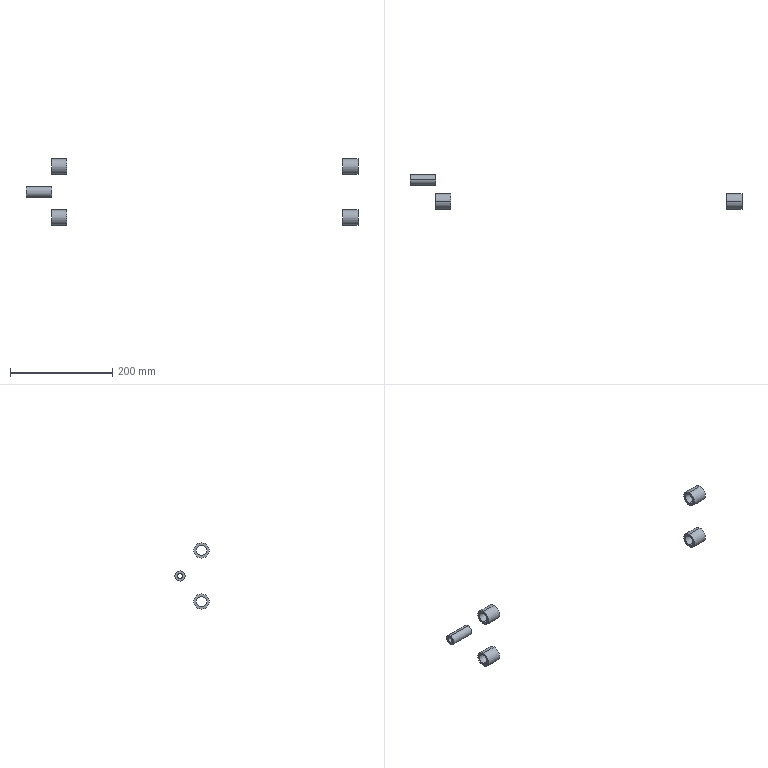Part | SolidWorks | features ICE 1, MirrorSolid 1, Revolution 1 | 5 solids | 30 faces | box 650 x 67 x 130 mm | volume 58905 mm3 | cylinder 20 | plane 10 | commonest cylinder face diameters 20 x10 30 x8 10 x2
STEP:
#1=CARTESIAN_POINT('',(-270.,0.,-10.));
#2=VERTEX_POINT('',#1);
#3=CARTESIAN_POINT('',(-270.,0.,10.));
#4=VERTEX_POINT('',#3);
#5=CARTESIAN_POINT('',(-270.,0.,0.));
#6=DIRECTION('',(-1.,0.,0.));
#7=DIRECTION('',(0.,0.,1.));
#8=AXIS2_PLACEMENT_3D('',#5,#6,#7);
#9=CIRCLE('',#8,10.);
#10=EDGE_CURVE('',#2,#4,#9,.T.);
#11=ORIENTED_EDGE('',*,*,#10,.F.);
#12=CARTESIAN_POINT('',(-300.,0.,-10.));
#13=VERTEX_POINT('',#12);
#14=CARTESIAN_POINT('',(-367.381,0.,-10.));
#15=DIRECTION('',(-1.,0.,0.));
#16=VECTOR('',#15,1000.);
#17=LINE('',#14,#16);
#18=EDGE_CURVE('',#2,#13,#17,.T.);
#19=ORIENTED_EDGE('',*,*,#18,.T.);
#20=CARTESIAN_POINT('',(-300.,0.,10.));
#21=VERTEX_POINT('',#20);
#22=CARTESIAN_POINT('',(-300.,0.,0.));
#23=DIRECTION('',(-1.,0.,0.));
#24=DIRECTION('',(0.,0.,1.));
#25=AXIS2_PLACEMENT_3D('',#22,#23,#24);
#26=CIRCLE('',#25,10.);
#27=EDGE_CURVE('',#13,#21,#26,.T.);
#28=ORIENTED_EDGE('',*,*,#27,.T.);
#29=CARTESIAN_POINT('',(-367.381,0.,10.));
#30=DIRECTION('',(-1.,0.,0.));
#31=VECTOR('',#30,1000.);
#32=LINE('',#29,#31);
#33=EDGE_CURVE('',#4,#21,#32,.T.);
#34=ORIENTED_EDGE('',*,*,#33,.F.);
#35=EDGE_LOOP('',(#11,#19,#28,#34));
#36=FACE_OUTER_BOUND('',#35,.T.);
#37=CARTESIAN_POINT('',(-367.381,0.,0.));
#38=DIRECTION('',(-1.,0.,0.));
#39=DIRECTION('',(0.,0.,1.));
#40=AXIS2_PLACEMENT_3D('',#37,#38,#39);
#41=CYLINDRICAL_SURFACE('',#40,10.);
#42=ADVANCED_FACE('',(#36),#41,.F.);
#43=CARTESIAN_POINT('',(-270.,0.,15.));
#44=VERTEX_POINT('',#43);
#45=CARTESIAN_POINT('',(-270.,0.,-15.));
#46=VERTEX_POINT('',#45);
#47=CARTESIAN_POINT('',(-270.,0.,0.));
#48=DIRECTION('',(-1.,0.,0.));
#49=DIRECTION('',(0.,0.,1.));
#50=AXIS2_PLACEMENT_3D('',#47,#48,#49);
#51=CIRCLE('',#50,15.);
#52=EDGE_CURVE('',#44,#46,#51,.T.);
#53=ORIENTED_EDGE('',*,*,#52,.T.);
#54=CARTESIAN_POINT('',(-300.,0.,-15.));
#55=VERTEX_POINT('',#54);
#56=CARTESIAN_POINT('',(-367.381,0.,-15.));
#57=DIRECTION('',(-1.,0.,0.));
#58=VECTOR('',#57,1000.);
#59=LINE('',#56,#58);
#60=EDGE_CURVE('',#46,#55,#59,.T.);
#61=ORIENTED_EDGE('',*,*,#60,.T.);
#62=CARTESIAN_POINT('',(-300.,0.,15.));
#63=VERTEX_POINT('',#62);
#64=CARTESIAN_POINT('',(-300.,0.,0.));
#65=DIRECTION('',(-1.,0.,0.));
#66=DIRECTION('',(0.,0.,1.));
#67=AXIS2_PLACEMENT_3D('',#64,#65,#66);
#68=CIRCLE('',#67,15.);
#69=EDGE_CURVE('',#63,#55,#68,.T.);
#70=ORIENTED_EDGE('',*,*,#69,.F.);
#71=CARTESIAN_POINT('',(-367.381,0.,15.));
#72=DIRECTION('',(-1.,0.,0.));
#73=VECTOR('',#72,1000.);
#74=LINE('',#71,#73);
#75=EDGE_CURVE('',#44,#63,#74,.T.);
#76=ORIENTED_EDGE('',*,*,#75,.F.);
#77=EDGE_LOOP('',(#53,#61,#70,#76));
#78=FACE_OUTER_BOUND('',#77,.T.);
#79=CARTESIAN_POINT('',(-367.381,0.,0.));
#80=DIRECTION('',(-1.,0.,0.));
#81=DIRECTION('',(0.,0.,1.));
#82=AXIS2_PLACEMENT_3D('',#79,#80,#81);
#83=CYLINDRICAL_SURFACE('',#82,15.);
#84=ADVANCED_FACE('',(#78),#83,.T.);
#85=ORIENTED_EDGE('',*,*,#60,.F.);
#86=CARTESIAN_POINT('',(-270.,0.,0.));
#87=DIRECTION('',(-1.,0.,0.));
#88=DIRECTION('',(0.,0.,1.));
#89=AXIS2_PLACEMENT_3D('',#86,#87,#88);
#90=CIRCLE('',#89,15.);
#91=EDGE_CURVE('',#46,#44,#90,.T.);
#92=ORIENTED_EDGE('',*,*,#91,.T.);
#93=ORIENTED_EDGE('',*,*,#75,.T.);
#94=CARTESIAN_POINT('',(-300.,0.,0.));
#95=DIRECTION('',(-1.,0.,0.));
#96=DIRECTION('',(0.,0.,1.));
#97=AXIS2_PLACEMENT_3D('',#94,#95,#96);
#98=CIRCLE('',#97,15.);
#99=EDGE_CURVE('',#55,#63,#98,.T.);
#100=ORIENTED_EDGE('',*,*,#99,.F.);
#101=EDGE_LOOP('',(#85,#92,#93,#100));
#102=FACE_OUTER_BOUND('',#101,.T.);
#103=CARTESIAN_POINT('',(-367.381,0.,0.));
#104=DIRECTION('',(-1.,0.,0.));
#105=DIRECTION('',(0.,0.,1.));
#106=AXIS2_PLACEMENT_3D('',#103,#104,#105);
#107=CYLINDRICAL_SURFACE('',#106,15.);
#108=ADVANCED_FACE('',(#102),#107,.T.);
#109=CARTESIAN_POINT('',(-300.,0.,0.));
#110=DIRECTION('',(-1.,0.,0.));
#111=DIRECTION('',(0.,0.,1.));
#112=AXIS2_PLACEMENT_3D('',#109,#110,#111);
#113=CIRCLE('',#112,10.);
#114=EDGE_CURVE('',#21,#13,#113,.T.);
#115=ORIENTED_EDGE('',*,*,#114,.F.);
#116=ORIENTED_EDGE('',*,*,#27,.F.);
#117=EDGE_LOOP('',(#115,#116));
#118=FACE_BOUND('',#117,.T.);
#119=ORIENTED_EDGE('',*,*,#69,.T.);
#120=ORIENTED_EDGE('',*,*,#99,.T.);
#121=EDGE_LOOP('',(#119,#120));
#122=FACE_OUTER_BOUND('',#121,.T.);
#123=CARTESIAN_POINT('',(-300.,15.,0.));
#124=DIRECTION('',(1.,0.,0.));
#125=DIRECTION('',(0.,0.,-1.));
#126=AXIS2_PLACEMENT_3D('',#123,#124,#125);
#127=PLANE('',#126);
#128=ADVANCED_FACE('',(#118,#122),#127,.F.);
#129=ORIENTED_EDGE('',*,*,#18,.F.);
#130=CARTESIAN_POINT('',(-270.,0.,0.));
#131=DIRECTION('',(-1.,0.,0.));
#132=DIRECTION('',(0.,0.,1.));
#133=AXIS2_PLACEMENT_3D('',#130,#131,#132);
#134=CIRCLE('',#133,10.);
#135=EDGE_CURVE('',#4,#2,#134,.T.);
#136=ORIENTED_EDGE('',*,*,#135,.F.);
#137=ORIENTED_EDGE('',*,*,#33,.T.);
#138=ORIENTED_EDGE('',*,*,#114,.T.);
#139=EDGE_LOOP('',(#129,#136,#137,#138));
#140=FACE_OUTER_BOUND('',#139,.T.);
#141=CARTESIAN_POINT('',(-367.381,0.,0.));
#142=DIRECTION('',(-1.,0.,0.));
#143=DIRECTION('',(0.,0.,1.));
#144=AXIS2_PLACEMENT_3D('',#141,#142,#143);
#145=CYLINDRICAL_SURFACE('',#144,10.);
#146=ADVANCED_FACE('',(#140),#145,.F.);
#147=ORIENTED_EDGE('',*,*,#52,.F.);
#148=ORIENTED_EDGE('',*,*,#91,.F.);
#149=EDGE_LOOP('',(#147,#148));
#150=FACE_OUTER_BOUND('',#149,.T.);
#151=ORIENTED_EDGE('',*,*,#135,.T.);
#152=ORIENTED_EDGE('',*,*,#10,.T.);
#153=EDGE_LOOP('',(#151,#152));
#154=FACE_BOUND('',#153,.T.);
#155=CARTESIAN_POINT('',(-270.,10.,0.));
#156=DIRECTION('',(-1.,0.,0.));
#157=DIRECTION('',(0.,0.,1.));
#158=AXIS2_PLACEMENT_3D('',#155,#156,#157);
#159=PLANE('',#158);
#160=ADVANCED_FACE('',(#150,#154),#159,.F.);
#161=CLOSED_SHELL('',(#42,#84,#108,#128,#146,#160));
#162=MANIFOLD_SOLID_BREP('',#161);
#163=CARTESIAN_POINT('',(300.,0.,-10.));
#164=VERTEX_POINT('',#163);
#165=CARTESIAN_POINT('',(300.,0.,10.));
#166=VERTEX_POINT('',#165);
#167=CARTESIAN_POINT('',(300.,0.,0.));
#168=DIRECTION('',(-1.,0.,0.));
#169=DIRECTION('',(0.,0.,1.));
#170=AXIS2_PLACEMENT_3D('',#167,#168,#169);
#171=CIRCLE('',#170,10.);
#172=EDGE_CURVE('',#164,#166,#171,.T.);
#173=ORIENTED_EDGE('',*,*,#172,.F.);
#174=CARTESIAN_POINT('',(270.,0.,-10.));
#175=VERTEX_POINT('',#174);
#176=CARTESIAN_POINT('',(-367.381,0.,-10.));
#177=DIRECTION('',(-1.,0.,0.));
#178=VECTOR('',#177,1000.);
#179=LINE('',#176,#178);
#180=EDGE_CURVE('',#164,#175,#179,.T.);
#181=ORIENTED_EDGE('',*,*,#180,.T.);
#182=CARTESIAN_POINT('',(270.,0.,10.));
#183=VERTEX_POINT('',#182);
#184=CARTESIAN_POINT('',(270.,0.,0.));
#185=DIRECTION('',(-1.,0.,0.));
#186=DIRECTION('',(0.,0.,1.));
#187=AXIS2_PLACEMENT_3D('',#184,#185,#186);
#188=CIRCLE('',#187,10.);
#189=EDGE_CURVE('',#175,#183,#188,.T.);
#190=ORIENTED_EDGE('',*,*,#189,.T.);
#191=CARTESIAN_POINT('',(-367.381,0.,10.));
#192=DIRECTION('',(-1.,0.,0.));
#193=VECTOR('',#192,1000.);
#194=LINE('',#191,#193);
#195=EDGE_CURVE('',#166,#183,#194,.T.);
#196=ORIENTED_EDGE('',*,*,#195,.F.);
#197=EDGE_LOOP('',(#173,#181,#190,#196));
#198=FACE_OUTER_BOUND('',#197,.T.);
#199=CARTESIAN_POINT('',(-367.381,0.,0.));
#200=DIRECTION('',(-1.,0.,0.));
#201=DIRECTION('',(0.,0.,1.));
#202=AXIS2_PLACEMENT_3D('',#199,#200,#201);
#203=CYLINDRICAL_SURFACE('',#202,10.);
#204=ADVANCED_FACE('',(#198),#203,.F.);
#205=CARTESIAN_POINT('',(300.,0.,15.));
#206=VERTEX_POINT('',#205);
#207=CARTESIAN_POINT('',(300.,0.,-15.));
#208=VERTEX_POINT('',#207);
#209=CARTESIAN_POINT('',(300.,0.,0.));
#210=DIRECTION('',(-1.,0.,0.));
#211=DIRECTION('',(0.,0.,1.));
#212=AXIS2_PLACEMENT_3D('',#209,#210,#211);
#213=CIRCLE('',#212,15.);
#214=EDGE_CURVE('',#206,#208,#213,.T.);
#215=ORIENTED_EDGE('',*,*,#214,.T.);
#216=CARTESIAN_POINT('',(270.,0.,-15.));
#217=VERTEX_POINT('',#216);
#218=CARTESIAN_POINT('',(-367.381,0.,-15.));
#219=DIRECTION('',(-1.,0.,0.));
#220=VECTOR('',#219,1000.);
#221=LINE('',#218,#220);
#222=EDGE_CURVE('',#208,#217,#221,.T.);
#223=ORIENTED_EDGE('',*,*,#222,.T.);
#224=CARTESIAN_POINT('',(270.,0.,15.));
#225=VERTEX_POINT('',#224);
#226=CARTESIAN_POINT('',(270.,0.,0.));
#227=DIRECTION('',(-1.,0.,0.));
#228=DIRECTION('',(0.,0.,1.));
#229=AXIS2_PLACEMENT_3D('',#226,#227,#228);
#230=CIRCLE('',#229,15.);
#231=EDGE_CURVE('',#225,#217,#230,.T.);
#232=ORIENTED_EDGE('',*,*,#231,.F.);
#233=CARTESIAN_POINT('',(-367.381,0.,15.));
#234=DIRECTION('',(-1.,0.,0.));
#235=VECTOR('',#234,1000.);
#236=LINE('',#233,#235);
#237=EDGE_CURVE('',#206,#225,#236,.T.);
#238=ORIENTED_EDGE('',*,*,#237,.F.);
#239=EDGE_LOOP('',(#215,#223,#232,#238));
#240=FACE_OUTER_BOUND('',#239,.T.);
#241=CARTESIAN_POINT('',(-367.381,0.,0.));
#242=DIRECTION('',(-1.,0.,0.));
#243=DIRECTION('',(0.,0.,1.));
#244=AXIS2_PLACEMENT_3D('',#241,#242,#243);
#245=CYLINDRICAL_SURFACE('',#244,15.);
#246=ADVANCED_FACE('',(#240),#245,.T.);
#247=ORIENTED_EDGE('',*,*,#222,.F.);
#248=CARTESIAN_POINT('',(300.,0.,0.));
#249=DIRECTION('',(-1.,0.,0.));
#250=DIRECTION('',(0.,0.,1.));
#251=AXIS2_PLACEMENT_3D('',#248,#249,#250);
#252=CIRCLE('',#251,15.);
#253=EDGE_CURVE('',#208,#206,#252,.T.);
#254=ORIENTED_EDGE('',*,*,#253,.T.);
#255=ORIENTED_EDGE('',*,*,#237,.T.);
#256=CARTESIAN_POINT('',(270.,0.,0.));
#257=DIRECTION('',(-1.,0.,0.));
#258=DIRECTION('',(0.,0.,1.));
#259=AXIS2_PLACEMENT_3D('',#256,#257,#258);
#260=CIRCLE('',#259,15.);
#261=EDGE_CURVE('',#217,#225,#260,.T.);
#262=ORIENTED_EDGE('',*,*,#261,.F.);
#263=EDGE_LOOP('',(#247,#254,#255,#262));
#264=FACE_OUTER_BOUND('',#263,.T.);
#265=CARTESIAN_POINT('',(-367.381,0.,0.));
#266=DIRECTION('',(-1.,0.,0.));
#267=DIRECTION('',(0.,0.,1.));
#268=AXIS2_PLACEMENT_3D('',#265,#266,#267);
#269=CYLINDRICAL_SURFACE('',#268,15.);
#270=ADVANCED_FACE('',(#264),#269,.T.);
#271=CARTESIAN_POINT('',(270.,0.,0.));
#272=DIRECTION('',(-1.,0.,0.));
#273=DIRECTION('',(0.,0.,1.));
#274=AXIS2_PLACEMENT_3D('',#271,#272,#273);
#275=CIRCLE('',#274,10.);
#276=EDGE_CURVE('',#183,#175,#275,.T.);
#277=ORIENTED_EDGE('',*,*,#276,.F.);
#278=ORIENTED_EDGE('',*,*,#189,.F.);
#279=EDGE_LOOP('',(#277,#278));
#280=FACE_BOUND('',#279,.T.);
#281=ORIENTED_EDGE('',*,*,#231,.T.);
#282=ORIENTED_EDGE('',*,*,#261,.T.);
#283=EDGE_LOOP('',(#281,#282));
#284=FACE_OUTER_BOUND('',#283,.T.);
#285=CARTESIAN_POINT('',(270.,15.,0.));
#286=DIRECTION('',(1.,0.,0.));
#287=DIRECTION('',(0.,0.,-1.));
#288=AXIS2_PLACEMENT_3D('',#285,#286,#287);
#289=PLANE('',#288);
#290=ADVANCED_FACE('',(#280,#284),#289,.F.);
#291=ORIENTED_EDGE('',*,*,#180,.F.);
#292=CARTESIAN_POINT('',(300.,0.,0.));
#293=DIRECTION('',(-1.,0.,0.));
#294=DIRECTION('',(0.,0.,1.));
#295=AXIS2_PLACEMENT_3D('',#292,#293,#294);
#296=CIRCLE('',#295,10.);
#297=EDGE_CURVE('',#166,#164,#296,.T.);
#298=ORIENTED_EDGE('',*,*,#297,.F.);
#299=ORIENTED_EDGE('',*,*,#195,.T.);
#300=ORIENTED_EDGE('',*,*,#276,.T.);
#301=EDGE_LOOP('',(#291,#298,#299,#300));
#302=FACE_OUTER_BOUND('',#301,.T.);
#303=CARTESIAN_POINT('',(-367.381,0.,0.));
#304=DIRECTION('',(-1.,0.,0.));
#305=DIRECTION('',(0.,0.,1.));
#306=AXIS2_PLACEMENT_3D('',#303,#304,#305);
#307=CYLINDRICAL_SURFACE('',#306,10.);
#308=ADVANCED_FACE('',(#302),#307,.F.);
#309=ORIENTED_EDGE('',*,*,#214,.F.);
#310=ORIENTED_EDGE('',*,*,#253,.F.);
#311=EDGE_LOOP('',(#309,#310));
#312=FACE_OUTER_BOUND('',#311,.T.);
#313=ORIENTED_EDGE('',*,*,#297,.T.);
#314=ORIENTED_EDGE('',*,*,#172,.T.);
#315=EDGE_LOOP('',(#313,#314));
#316=FACE_BOUND('',#315,.T.);
#317=CARTESIAN_POINT('',(300.,10.,0.));
#318=DIRECTION('',(-1.,0.,0.));
#319=DIRECTION('',(0.,0.,1.));
#320=AXIS2_PLACEMENT_3D('',#317,#318,#319);
#321=PLANE('',#320);
#322=ADVANCED_FACE('',(#312,#316),#321,.F.);
#323=CLOSED_SHELL('',(#204,#246,#270,#290,#308,#322));
#324=MANIFOLD_SOLID_BREP('',#323);
#325=CARTESIAN_POINT('',(-270.,0.,90.));
#326=VERTEX_POINT('',#325);
#327=CARTESIAN_POINT('',(-270.,0.,110.));
#328=VERTEX_POINT('',#327);
#329=CARTESIAN_POINT('',(-270.,0.,100.));
#330=DIRECTION('',(1.,0.,0.));
#331=DIRECTION('',(0.,0.,-1.));
#332=AXIS2_PLACEMENT_3D('',#329,#330,#331);
#333=CIRCLE('',#332,10.);
#334=EDGE_CURVE('',#326,#328,#333,.T.);
#335=ORIENTED_EDGE('',*,*,#334,.T.);
#336=CARTESIAN_POINT('',(-300.,0.,110.));
#337=VERTEX_POINT('',#336);
#338=CARTESIAN_POINT('',(-367.381,0.,110.));
#339=DIRECTION('',(-1.,0.,0.));
#340=VECTOR('',#339,1000.);
#341=LINE('',#338,#340);
#342=EDGE_CURVE('',#328,#337,#341,.T.);
#343=ORIENTED_EDGE('',*,*,#342,.T.);
#344=CARTESIAN_POINT('',(-300.,0.,90.));
#345=VERTEX_POINT('',#344);
#346=CARTESIAN_POINT('',(-300.,0.,100.));
#347=DIRECTION('',(1.,0.,0.));
#348=DIRECTION('',(0.,0.,-1.));
#349=AXIS2_PLACEMENT_3D('',#346,#347,#348);
#350=CIRCLE('',#349,10.);
#351=EDGE_CURVE('',#345,#337,#350,.T.);
#352=ORIENTED_EDGE('',*,*,#351,.F.);
#353=CARTESIAN_POINT('',(-367.381,0.,90.));
#354=DIRECTION('',(-1.,0.,0.));
#355=VECTOR('',#354,1000.);
#356=LINE('',#353,#355);
#357=EDGE_CURVE('',#326,#345,#356,.T.);
#358=ORIENTED_EDGE('',*,*,#357,.F.);
#359=EDGE_LOOP('',(#335,#343,#352,#358));
#360=FACE_OUTER_BOUND('',#359,.T.);
#361=CARTESIAN_POINT('',(-367.381,0.,100.));
#362=DIRECTION('',(-1.,0.,0.));
#363=DIRECTION('',(0.,0.,-1.));
#364=AXIS2_PLACEMENT_3D('',#361,#362,#363);
#365=CYLINDRICAL_SURFACE('',#364,10.);
#366=ADVANCED_FACE('',(#360),#365,.F.);
#367=CARTESIAN_POINT('',(-270.,0.,115.));
#368=VERTEX_POINT('',#367);
#369=CARTESIAN_POINT('',(-270.,0.,85.));
#370=VERTEX_POINT('',#369);
#371=CARTESIAN_POINT('',(-270.,0.,100.));
#372=DIRECTION('',(1.,0.,0.));
#373=DIRECTION('',(0.,0.,-1.));
#374=AXIS2_PLACEMENT_3D('',#371,#372,#373);
#375=CIRCLE('',#374,15.);
#376=EDGE_CURVE('',#368,#370,#375,.T.);
#377=ORIENTED_EDGE('',*,*,#376,.F.);
#378=CARTESIAN_POINT('',(-300.,0.,115.));
#379=VERTEX_POINT('',#378);
#380=CARTESIAN_POINT('',(-367.381,0.,115.));
#381=DIRECTION('',(-1.,0.,0.));
#382=VECTOR('',#381,1000.);
#383=LINE('',#380,#382);
#384=EDGE_CURVE('',#368,#379,#383,.T.);
#385=ORIENTED_EDGE('',*,*,#384,.T.);
#386=CARTESIAN_POINT('',(-300.,0.,85.));
#387=VERTEX_POINT('',#386);
#388=CARTESIAN_POINT('',(-300.,0.,100.));
#389=DIRECTION('',(1.,0.,0.));
#390=DIRECTION('',(0.,0.,-1.));
#391=AXIS2_PLACEMENT_3D('',#388,#389,#390);
#392=CIRCLE('',#391,15.);
#393=EDGE_CURVE('',#379,#387,#392,.T.);
#394=ORIENTED_EDGE('',*,*,#393,.T.);
#395=CARTESIAN_POINT('',(-367.381,0.,85.));
#396=DIRECTION('',(-1.,0.,0.));
#397=VECTOR('',#396,1000.);
#398=LINE('',#395,#397);
#399=EDGE_CURVE('',#370,#387,#398,.T.);
#400=ORIENTED_EDGE('',*,*,#399,.F.);
#401=EDGE_LOOP('',(#377,#385,#394,#400));
#402=FACE_OUTER_BOUND('',#401,.T.);
#403=CARTESIAN_POINT('',(-367.381,0.,100.));
#404=DIRECTION('',(-1.,0.,0.));
#405=DIRECTION('',(0.,0.,-1.));
#406=AXIS2_PLACEMENT_3D('',#403,#404,#405);
#407=CYLINDRICAL_SURFACE('',#406,15.);
#408=ADVANCED_FACE('',(#402),#407,.T.);
#409=ORIENTED_EDGE('',*,*,#384,.F.);
#410=CARTESIAN_POINT('',(-270.,0.,100.));
#411=DIRECTION('',(1.,0.,0.));
#412=DIRECTION('',(0.,0.,-1.));
#413=AXIS2_PLACEMENT_3D('',#410,#411,#412);
#414=CIRCLE('',#413,15.);
#415=EDGE_CURVE('',#370,#368,#414,.T.);
#416=ORIENTED_EDGE('',*,*,#415,.F.);
#417=ORIENTED_EDGE('',*,*,#399,.T.);
#418=CARTESIAN_POINT('',(-300.,0.,100.));
#419=DIRECTION('',(1.,0.,0.));
#420=DIRECTION('',(0.,0.,-1.));
#421=AXIS2_PLACEMENT_3D('',#418,#419,#420);
#422=CIRCLE('',#421,15.);
#423=EDGE_CURVE('',#387,#379,#422,.T.);
#424=ORIENTED_EDGE('',*,*,#423,.T.);
#425=EDGE_LOOP('',(#409,#416,#417,#424));
#426=FACE_OUTER_BOUND('',#425,.T.);
#427=CARTESIAN_POINT('',(-367.381,0.,100.));
#428=DIRECTION('',(-1.,0.,0.));
#429=DIRECTION('',(0.,0.,-1.));
#430=AXIS2_PLACEMENT_3D('',#427,#428,#429);
#431=CYLINDRICAL_SURFACE('',#430,15.);
#432=ADVANCED_FACE('',(#426),#431,.T.);
#433=ORIENTED_EDGE('',*,*,#351,.T.);
#434=CARTESIAN_POINT('',(-300.,0.,100.));
#435=DIRECTION('',(1.,0.,0.));
#436=DIRECTION('',(0.,0.,-1.));
#437=AXIS2_PLACEMENT_3D('',#434,#435,#436);
#438=CIRCLE('',#437,10.);
#439=EDGE_CURVE('',#337,#345,#438,.T.);
#440=ORIENTED_EDGE('',*,*,#439,.T.);
#441=EDGE_LOOP('',(#433,#440));
#442=FACE_BOUND('',#441,.T.);
#443=ORIENTED_EDGE('',*,*,#423,.F.);
#444=ORIENTED_EDGE('',*,*,#393,.F.);
#445=EDGE_LOOP('',(#443,#444));
#446=FACE_OUTER_BOUND('',#445,.T.);
#447=CARTESIAN_POINT('',(-300.,15.,100.));
#448=DIRECTION('',(1.,0.,0.));
#449=DIRECTION('',(0.,0.,1.));
#450=AXIS2_PLACEMENT_3D('',#447,#448,#449);
#451=PLANE('',#450);
#452=ADVANCED_FACE('',(#442,#446),#451,.F.);
#453=ORIENTED_EDGE('',*,*,#342,.F.);
#454=CARTESIAN_POINT('',(-270.,0.,100.));
#455=DIRECTION('',(1.,0.,0.));
#456=DIRECTION('',(0.,0.,-1.));
#457=AXIS2_PLACEMENT_3D('',#454,#455,#456);
#458=CIRCLE('',#457,10.);
#459=EDGE_CURVE('',#328,#326,#458,.T.);
#460=ORIENTED_EDGE('',*,*,#459,.T.);
#461=ORIENTED_EDGE('',*,*,#357,.T.);
#462=ORIENTED_EDGE('',*,*,#439,.F.);
#463=EDGE_LOOP('',(#453,#460,#461,#462));
#464=FACE_OUTER_BOUND('',#463,.T.);
#465=CARTESIAN_POINT('',(-367.381,0.,100.));
#466=DIRECTION('',(-1.,0.,0.));
#467=DIRECTION('',(0.,0.,-1.));
#468=AXIS2_PLACEMENT_3D('',#465,#466,#467);
#469=CYLINDRICAL_SURFACE('',#468,10.);
#470=ADVANCED_FACE('',(#464),#469,.F.);
#471=ORIENTED_EDGE('',*,*,#415,.T.);
#472=ORIENTED_EDGE('',*,*,#376,.T.);
#473=EDGE_LOOP('',(#471,#472));
#474=FACE_OUTER_BOUND('',#473,.T.);
#475=ORIENTED_EDGE('',*,*,#334,.F.);
#476=ORIENTED_EDGE('',*,*,#459,.F.);
#477=EDGE_LOOP('',(#475,#476));
#478=FACE_BOUND('',#477,.T.);
#479=CARTESIAN_POINT('',(-270.,10.,100.));
#480=DIRECTION('',(-1.,0.,0.));
#481=DIRECTION('',(0.,0.,-1.));
#482=AXIS2_PLACEMENT_3D('',#479,#480,#481);
#483=PLANE('',#482);
#484=ADVANCED_FACE('',(#474,#478),#483,.F.);
#485=CLOSED_SHELL('',(#366,#408,#432,#452,#470,#484));
#486=MANIFOLD_SOLID_BREP('',#485);
#487=CARTESIAN_POINT('',(300.,0.,90.));
#488=VERTEX_POINT('',#487);
#489=CARTESIAN_POINT('',(300.,0.,110.));
#490=VERTEX_POINT('',#489);
#491=CARTESIAN_POINT('',(300.,0.,100.));
#492=DIRECTION('',(1.,0.,0.));
#493=DIRECTION('',(0.,0.,-1.));
#494=AXIS2_PLACEMENT_3D('',#491,#492,#493);
#495=CIRCLE('',#494,10.);
#496=EDGE_CURVE('',#488,#490,#495,.T.);
#497=ORIENTED_EDGE('',*,*,#496,.T.);
#498=CARTESIAN_POINT('',(270.,0.,110.));
#499=VERTEX_POINT('',#498);
#500=CARTESIAN_POINT('',(-367.381,0.,110.));
#501=DIRECTION('',(-1.,0.,0.));
#502=VECTOR('',#501,1000.);
#503=LINE('',#500,#502);
#504=EDGE_CURVE('',#490,#499,#503,.T.);
#505=ORIENTED_EDGE('',*,*,#504,.T.);
#506=CARTESIAN_POINT('',(270.,0.,90.));
#507=VERTEX_POINT('',#506);
#508=CARTESIAN_POINT('',(270.,0.,100.));
#509=DIRECTION('',(1.,0.,0.));
#510=DIRECTION('',(0.,0.,-1.));
#511=AXIS2_PLACEMENT_3D('',#508,#509,#510);
#512=CIRCLE('',#511,10.);
#513=EDGE_CURVE('',#507,#499,#512,.T.);
#514=ORIENTED_EDGE('',*,*,#513,.F.);
#515=CARTESIAN_POINT('',(-367.381,0.,90.));
#516=DIRECTION('',(-1.,0.,0.));
#517=VECTOR('',#516,1000.);
#518=LINE('',#515,#517);
#519=EDGE_CURVE('',#488,#507,#518,.T.);
#520=ORIENTED_EDGE('',*,*,#519,.F.);
#521=EDGE_LOOP('',(#497,#505,#514,#520));
#522=FACE_OUTER_BOUND('',#521,.T.);
#523=CARTESIAN_POINT('',(-367.381,0.,100.));
#524=DIRECTION('',(-1.,0.,0.));
#525=DIRECTION('',(0.,0.,-1.));
#526=AXIS2_PLACEMENT_3D('',#523,#524,#525);
#527=CYLINDRICAL_SURFACE('',#526,10.);
#528=ADVANCED_FACE('',(#522),#527,.F.);
#529=CARTESIAN_POINT('',(300.,0.,115.));
#530=VERTEX_POINT('',#529);
#531=CARTESIAN_POINT('',(300.,0.,85.));
#532=VERTEX_POINT('',#531);
#533=CARTESIAN_POINT('',(300.,0.,100.));
#534=DIRECTION('',(1.,0.,0.));
#535=DIRECTION('',(0.,0.,-1.));
#536=AXIS2_PLACEMENT_3D('',#533,#534,#535);
#537=CIRCLE('',#536,15.);
#538=EDGE_CURVE('',#530,#532,#537,.T.);
#539=ORIENTED_EDGE('',*,*,#538,.F.);
#540=CARTESIAN_POINT('',(270.,0.,115.));
#541=VERTEX_POINT('',#540);
#542=CARTESIAN_POINT('',(-367.381,0.,115.));
#543=DIRECTION('',(-1.,0.,0.));
#544=VECTOR('',#543,1000.);
#545=LINE('',#542,#544);
#546=EDGE_CURVE('',#530,#541,#545,.T.);
#547=ORIENTED_EDGE('',*,*,#546,.T.);
#548=CARTESIAN_POINT('',(270.,0.,85.));
#549=VERTEX_POINT('',#548);
#550=CARTESIAN_POINT('',(270.,0.,100.));
#551=DIRECTION('',(1.,0.,0.));
#552=DIRECTION('',(0.,0.,-1.));
#553=AXIS2_PLACEMENT_3D('',#550,#551,#552);
#554=CIRCLE('',#553,15.);
#555=EDGE_CURVE('',#541,#549,#554,.T.);
#556=ORIENTED_EDGE('',*,*,#555,.T.);
#557=CARTESIAN_POINT('',(-367.381,0.,85.));
#558=DIRECTION('',(-1.,0.,0.));
#559=VECTOR('',#558,1000.);
#560=LINE('',#557,#559);
#561=EDGE_CURVE('',#532,#549,#560,.T.);
#562=ORIENTED_EDGE('',*,*,#561,.F.);
#563=EDGE_LOOP('',(#539,#547,#556,#562));
#564=FACE_OUTER_BOUND('',#563,.T.);
#565=CARTESIAN_POINT('',(-367.381,0.,100.));
#566=DIRECTION('',(-1.,0.,0.));
#567=DIRECTION('',(0.,0.,-1.));
#568=AXIS2_PLACEMENT_3D('',#565,#566,#567);
#569=CYLINDRICAL_SURFACE('',#568,15.);
#570=ADVANCED_FACE('',(#564),#569,.T.);
#571=ORIENTED_EDGE('',*,*,#546,.F.);
#572=CARTESIAN_POINT('',(300.,0.,100.));
#573=DIRECTION('',(1.,0.,0.));
#574=DIRECTION('',(0.,0.,-1.));
#575=AXIS2_PLACEMENT_3D('',#572,#573,#574);
#576=CIRCLE('',#575,15.);
#577=EDGE_CURVE('',#532,#530,#576,.T.);
#578=ORIENTED_EDGE('',*,*,#577,.F.);
#579=ORIENTED_EDGE('',*,*,#561,.T.);
#580=CARTESIAN_POINT('',(270.,0.,100.));
#581=DIRECTION('',(1.,0.,0.));
#582=DIRECTION('',(0.,0.,-1.));
#583=AXIS2_PLACEMENT_3D('',#580,#581,#582);
#584=CIRCLE('',#583,15.);
#585=EDGE_CURVE('',#549,#541,#584,.T.);
#586=ORIENTED_EDGE('',*,*,#585,.T.);
#587=EDGE_LOOP('',(#571,#578,#579,#586));
#588=FACE_OUTER_BOUND('',#587,.T.);
#589=CARTESIAN_POINT('',(-367.381,0.,100.));
#590=DIRECTION('',(-1.,0.,0.));
#591=DIRECTION('',(0.,0.,-1.));
#592=AXIS2_PLACEMENT_3D('',#589,#590,#591);
#593=CYLINDRICAL_SURFACE('',#592,15.);
#594=ADVANCED_FACE('',(#588),#593,.T.);
#595=ORIENTED_EDGE('',*,*,#513,.T.);
#596=CARTESIAN_POINT('',(270.,0.,100.));
#597=DIRECTION('',(1.,0.,0.));
#598=DIRECTION('',(0.,0.,-1.));
#599=AXIS2_PLACEMENT_3D('',#596,#597,#598);
#600=CIRCLE('',#599,10.);
#601=EDGE_CURVE('',#499,#507,#600,.T.);
#602=ORIENTED_EDGE('',*,*,#601,.T.);
#603=EDGE_LOOP('',(#595,#602));
#604=FACE_BOUND('',#603,.T.);
#605=ORIENTED_EDGE('',*,*,#585,.F.);
#606=ORIENTED_EDGE('',*,*,#555,.F.);
#607=EDGE_LOOP('',(#605,#606));
#608=FACE_OUTER_BOUND('',#607,.T.);
#609=CARTESIAN_POINT('',(270.,15.,100.));
#610=DIRECTION('',(1.,0.,0.));
#611=DIRECTION('',(0.,0.,1.));
#612=AXIS2_PLACEMENT_3D('',#609,#610,#611);
#613=PLANE('',#612);
#614=ADVANCED_FACE('',(#604,#608),#613,.F.);
#615=ORIENTED_EDGE('',*,*,#504,.F.);
#616=CARTESIAN_POINT('',(300.,0.,100.));
#617=DIRECTION('',(1.,0.,0.));
#618=DIRECTION('',(0.,0.,-1.));
#619=AXIS2_PLACEMENT_3D('',#616,#617,#618);
#620=CIRCLE('',#619,10.);
#621=EDGE_CURVE('',#490,#488,#620,.T.);
#622=ORIENTED_EDGE('',*,*,#621,.T.);
#623=ORIENTED_EDGE('',*,*,#519,.T.);
#624=ORIENTED_EDGE('',*,*,#601,.F.);
#625=EDGE_LOOP('',(#615,#622,#623,#624));
#626=FACE_OUTER_BOUND('',#625,.T.);
#627=CARTESIAN_POINT('',(-367.381,0.,100.));
#628=DIRECTION('',(-1.,0.,0.));
#629=DIRECTION('',(0.,0.,-1.));
#630=AXIS2_PLACEMENT_3D('',#627,#628,#629);
#631=CYLINDRICAL_SURFACE('',#630,10.);
#632=ADVANCED_FACE('',(#626),#631,.F.);
#633=ORIENTED_EDGE('',*,*,#577,.T.);
#634=ORIENTED_EDGE('',*,*,#538,.T.);
#635=EDGE_LOOP('',(#633,#634));
#636=FACE_OUTER_BOUND('',#635,.T.);
#637=ORIENTED_EDGE('',*,*,#496,.F.);
#638=ORIENTED_EDGE('',*,*,#621,.F.);
#639=EDGE_LOOP('',(#637,#638));
#640=FACE_BOUND('',#639,.T.);
#641=CARTESIAN_POINT('',(300.,10.,100.));
#642=DIRECTION('',(-1.,0.,0.));
#643=DIRECTION('',(0.,0.,-1.));
#644=AXIS2_PLACEMENT_3D('',#641,#642,#643);
#645=PLANE('',#644);
#646=ADVANCED_FACE('',(#636,#640),#645,.F.);
#647=CLOSED_SHELL('',(#528,#570,#594,#614,#632,#646));
#648=MANIFOLD_SOLID_BREP('',#647);
#649=CARTESIAN_POINT('',(-350.,42.,45.));
#650=VERTEX_POINT('',#649);
#651=CARTESIAN_POINT('',(-350.,42.,55.));
#652=VERTEX_POINT('',#651);
#653=CARTESIAN_POINT('',(-350.,42.,50.));
#654=DIRECTION('',(-1.,0.,0.));
#655=DIRECTION('',(0.,0.,1.));
#656=AXIS2_PLACEMENT_3D('',#653,#654,#655);
#657=CIRCLE('',#656,5.);
#658=EDGE_CURVE('',#650,#652,#657,.T.);
#659=ORIENTED_EDGE('',*,*,#658,.T.);
#660=CARTESIAN_POINT('',(-300.,42.,55.));
#661=VERTEX_POINT('',#660);
#662=CARTESIAN_POINT('',(-350.,42.,55.));
#663=DIRECTION('',(1.,0.,0.));
#664=VECTOR('',#663,1000.);
#665=LINE('',#662,#664);
#666=EDGE_CURVE('',#652,#661,#665,.T.);
#667=ORIENTED_EDGE('',*,*,#666,.T.);
#668=CARTESIAN_POINT('',(-300.,42.,45.));
#669=VERTEX_POINT('',#668);
#670=CARTESIAN_POINT('',(-300.,42.,50.));
#671=DIRECTION('',(-1.,0.,0.));
#672=DIRECTION('',(0.,0.,1.));
#673=AXIS2_PLACEMENT_3D('',#670,#671,#672);
#674=CIRCLE('',#673,5.);
#675=EDGE_CURVE('',#669,#661,#674,.T.);
#676=ORIENTED_EDGE('',*,*,#675,.F.);
#677=CARTESIAN_POINT('',(-350.,42.,45.));
#678=DIRECTION('',(1.,0.,0.));
#679=VECTOR('',#678,1000.);
#680=LINE('',#677,#679);
#681=EDGE_CURVE('',#650,#669,#680,.T.);
#682=ORIENTED_EDGE('',*,*,#681,.F.);
#683=EDGE_LOOP('',(#659,#667,#676,#682));
#684=FACE_OUTER_BOUND('',#683,.T.);
#685=CARTESIAN_POINT('',(-350.,42.,50.));
#686=DIRECTION('',(1.,0.,0.));
#687=DIRECTION('',(0.,0.,-1.));
#688=AXIS2_PLACEMENT_3D('',#685,#686,#687);
#689=CYLINDRICAL_SURFACE('',#688,5.);
#690=ADVANCED_FACE('',(#684),#689,.F.);
#691=CARTESIAN_POINT('',(-350.,42.,60.));
#692=VERTEX_POINT('',#691);
#693=CARTESIAN_POINT('',(-350.,42.,40.));
#694=VERTEX_POINT('',#693);
#695=CARTESIAN_POINT('',(-350.,42.,50.));
#696=DIRECTION('',(-1.,0.,0.));
#697=DIRECTION('',(0.,0.,1.));
#698=AXIS2_PLACEMENT_3D('',#695,#696,#697);
#699=CIRCLE('',#698,10.);
#700=EDGE_CURVE('',#692,#694,#699,.T.);
#701=ORIENTED_EDGE('',*,*,#700,.F.);
#702=CARTESIAN_POINT('',(-300.,42.,60.));
#703=VERTEX_POINT('',#702);
#704=CARTESIAN_POINT('',(-350.,42.,60.));
#705=DIRECTION('',(1.,0.,0.));
#706=VECTOR('',#705,1000.);
#707=LINE('',#704,#706);
#708=EDGE_CURVE('',#692,#703,#707,.T.);
#709=ORIENTED_EDGE('',*,*,#708,.T.);
#710=CARTESIAN_POINT('',(-300.,42.,40.));
#711=VERTEX_POINT('',#710);
#712=CARTESIAN_POINT('',(-300.,42.,50.));
#713=DIRECTION('',(-1.,0.,0.));
#714=DIRECTION('',(0.,0.,1.));
#715=AXIS2_PLACEMENT_3D('',#712,#713,#714);
#716=CIRCLE('',#715,10.);
#717=EDGE_CURVE('',#703,#711,#716,.T.);
#718=ORIENTED_EDGE('',*,*,#717,.T.);
#719=CARTESIAN_POINT('',(-350.,42.,40.));
#720=DIRECTION('',(1.,0.,0.));
#721=VECTOR('',#720,1000.);
#722=LINE('',#719,#721);
#723=EDGE_CURVE('',#694,#711,#722,.T.);
#724=ORIENTED_EDGE('',*,*,#723,.F.);
#725=EDGE_LOOP('',(#701,#709,#718,#724));
#726=FACE_OUTER_BOUND('',#725,.T.);
#727=CARTESIAN_POINT('',(-350.,42.,50.));
#728=DIRECTION('',(1.,0.,0.));
#729=DIRECTION('',(0.,0.,-1.));
#730=AXIS2_PLACEMENT_3D('',#727,#728,#729);
#731=CYLINDRICAL_SURFACE('',#730,10.);
#732=ADVANCED_FACE('',(#726),#731,.T.);
#733=CARTESIAN_POINT('',(-350.,42.,50.));
#734=DIRECTION('',(-1.,0.,0.));
#735=DIRECTION('',(0.,0.,1.));
#736=AXIS2_PLACEMENT_3D('',#733,#734,#735);
#737=CIRCLE('',#736,10.);
#738=EDGE_CURVE('',#694,#692,#737,.T.);
#739=ORIENTED_EDGE('',*,*,#738,.T.);
#740=ORIENTED_EDGE('',*,*,#700,.T.);
#741=EDGE_LOOP('',(#739,#740));
#742=FACE_OUTER_BOUND('',#741,.T.);
#743=ORIENTED_EDGE('',*,*,#658,.F.);
#744=CARTESIAN_POINT('',(-350.,42.,50.));
#745=DIRECTION('',(-1.,0.,0.));
#746=DIRECTION('',(0.,0.,1.));
#747=AXIS2_PLACEMENT_3D('',#744,#745,#746);
#748=CIRCLE('',#747,5.);
#749=EDGE_CURVE('',#652,#650,#748,.T.);
#750=ORIENTED_EDGE('',*,*,#749,.F.);
#751=EDGE_LOOP('',(#743,#750));
#752=FACE_BOUND('',#751,.T.);
#753=CARTESIAN_POINT('',(-350.,42.,50.));
#754=DIRECTION('',(-1.,0.,0.));
#755=DIRECTION('',(0.,0.,1.));
#756=AXIS2_PLACEMENT_3D('',#753,#754,#755);
#757=PLANE('',#756);
#758=ADVANCED_FACE('',(#742,#752),#757,.T.);
#759=CARTESIAN_POINT('',(-300.,42.,50.));
#760=DIRECTION('',(-1.,0.,0.));
#761=DIRECTION('',(0.,0.,1.));
#762=AXIS2_PLACEMENT_3D('',#759,#760,#761);
#763=CIRCLE('',#762,10.);
#764=EDGE_CURVE('',#711,#703,#763,.T.);
#765=ORIENTED_EDGE('',*,*,#764,.F.);
#766=ORIENTED_EDGE('',*,*,#717,.F.);
#767=EDGE_LOOP('',(#765,#766));
#768=FACE_OUTER_BOUND('',#767,.T.);
#769=ORIENTED_EDGE('',*,*,#675,.T.);
#770=CARTESIAN_POINT('',(-300.,42.,50.));
#771=DIRECTION('',(-1.,0.,0.));
#772=DIRECTION('',(0.,0.,1.));
#773=AXIS2_PLACEMENT_3D('',#770,#771,#772);
#774=CIRCLE('',#773,5.);
#775=EDGE_CURVE('',#661,#669,#774,.T.);
#776=ORIENTED_EDGE('',*,*,#775,.T.);
#777=EDGE_LOOP('',(#769,#776));
#778=FACE_BOUND('',#777,.T.);
#779=CARTESIAN_POINT('',(-300.,42.,50.));
#780=DIRECTION('',(-1.,0.,0.));
#781=DIRECTION('',(0.,0.,1.));
#782=AXIS2_PLACEMENT_3D('',#779,#780,#781);
#783=PLANE('',#782);
#784=ADVANCED_FACE('',(#768,#778),#783,.F.);
#785=ORIENTED_EDGE('',*,*,#708,.F.);
#786=ORIENTED_EDGE('',*,*,#738,.F.);
#787=ORIENTED_EDGE('',*,*,#723,.T.);
#788=ORIENTED_EDGE('',*,*,#764,.T.);
#789=EDGE_LOOP('',(#785,#786,#787,#788));
#790=FACE_OUTER_BOUND('',#789,.T.);
#791=CARTESIAN_POINT('',(-350.,42.,50.));
#792=DIRECTION('',(1.,0.,0.));
#793=DIRECTION('',(0.,0.,-1.));
#794=AXIS2_PLACEMENT_3D('',#791,#792,#793);
#795=CYLINDRICAL_SURFACE('',#794,10.);
#796=ADVANCED_FACE('',(#790),#795,.T.);
#797=ORIENTED_EDGE('',*,*,#666,.F.);
#798=ORIENTED_EDGE('',*,*,#749,.T.);
#799=ORIENTED_EDGE('',*,*,#681,.T.);
#800=ORIENTED_EDGE('',*,*,#775,.F.);
#801=EDGE_LOOP('',(#797,#798,#799,#800));
#802=FACE_OUTER_BOUND('',#801,.T.);
#803=CARTESIAN_POINT('',(-350.,42.,50.));
#804=DIRECTION('',(1.,0.,0.));
#805=DIRECTION('',(0.,0.,-1.));
#806=AXIS2_PLACEMENT_3D('',#803,#804,#805);
#807=CYLINDRICAL_SURFACE('',#806,5.);
#808=ADVANCED_FACE('',(#802),#807,.F.);
#809=CLOSED_SHELL('',(#690,#732,#758,#784,#796,#808));
#810=MANIFOLD_SOLID_BREP('',#809);
#811=CARTESIAN_POINT('',(0.,0.,0.));
#812=DIRECTION('',(0.,0.,1.));
#813=DIRECTION('',(1.,0.,0.));
#814=AXIS2_PLACEMENT_3D('',#811,#812,#813);
#815=(LENGTH_UNIT()NAMED_UNIT(*)SI_UNIT(.MILLI.,.METRE.));
#816=UNCERTAINTY_MEASURE_WITH_UNIT(LENGTH_MEASURE(0.00001),#815,'','');
#817=(NAMED_UNIT(*)PLANE_ANGLE_UNIT()SI_UNIT($,.RADIAN.));
#818=(NAMED_UNIT(*)SI_UNIT($,.STERADIAN.)SOLID_ANGLE_UNIT());
#819=(GEOMETRIC_REPRESENTATION_CONTEXT(3)GLOBAL_UNCERTAINTY_ASSIGNED_CONTEXT((#816))GLOBAL_UNIT_ASSIGNED_CONTEXT((#815,#817,#818))REPRESENTATION_CONTEXT('',''));
#820=ADVANCED_BREP_SHAPE_REPRESENTATION('',(#162,#324,#486,#648,#810,#814),#819);